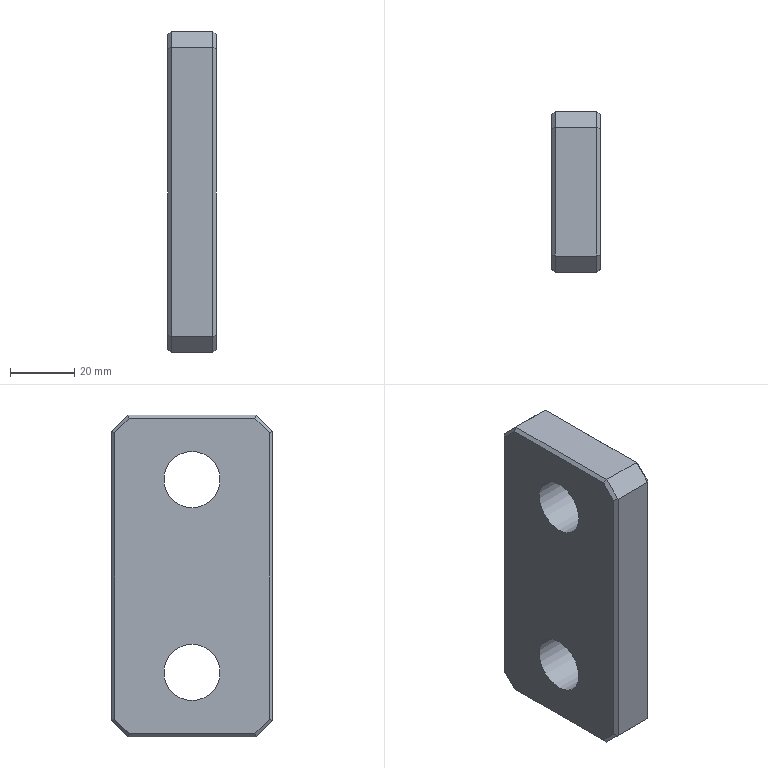Part | STEP file | solid 37 | 1 solid | 28 faces | box 15 x 50 x 100 mm | volume 66748 mm3 | plane 26 | cylinder 2 | commonest cylinder face diameters 17.5 x2